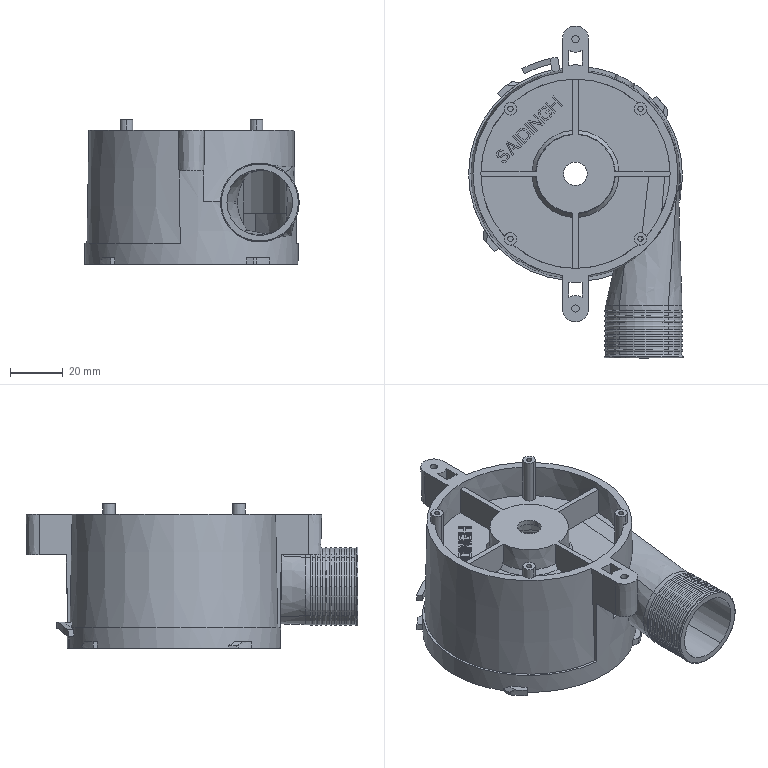Part | STEP file | BENG1118_AF0_35_2_1_1 | 1 solid | 412 faces | box 81.69 x 126.25 x 55 mm | volume 61777 mm3 | plane 260 | cylinder 84 | cone 38 | torus 20 | spline 10 | commonest cylinder face diameters 28.999 x20 29 x20 2 x8 4.8 x8 2.8 x4 3 x4